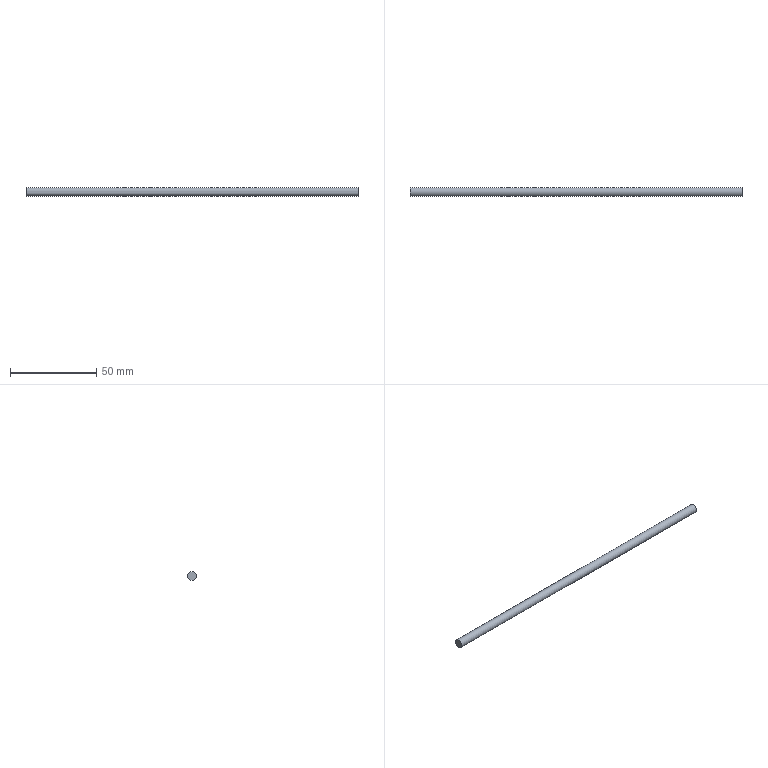Part | NX | features solid 2 | 1 solid | 3 faces | box 192 x 5 x 5 mm | volume 3770 mm3 | plane 2 | cylinder 1 | commonest cylinder face diameters 5 x1
STEP:
#1=CARTESIAN_POINT('',(-65.,-377.5,-412.5));
#2=VERTEX_POINT('',#1);
#3=CARTESIAN_POINT('',(-65.,-377.5,-410.));
#4=DIRECTION('',(1.,0.,0.));
#5=DIRECTION('',(0.,0.,-1.));
#6=AXIS2_PLACEMENT_3D('',#3,#4,#5);
#7=CIRCLE('',#6,2.5);
#8=EDGE_CURVE('',#2,#2,#7,.T.);
#9=ORIENTED_EDGE('',*,*,#8,.F.);
#10=EDGE_LOOP('',(#9));
#11=FACE_BOUND('',#10,.T.);
#12=CARTESIAN_POINT('',(-257.,-377.5,-412.5));
#13=VERTEX_POINT('',#12);
#14=CARTESIAN_POINT('',(-257.,-377.5,-410.));
#15=DIRECTION('',(1.,0.,0.));
#16=DIRECTION('',(0.,0.,-1.));
#17=AXIS2_PLACEMENT_3D('',#14,#15,#16);
#18=CIRCLE('',#17,2.5);
#19=EDGE_CURVE('',#13,#13,#18,.T.);
#20=ORIENTED_EDGE('',*,*,#19,.T.);
#21=EDGE_LOOP('',(#20));
#22=FACE_BOUND('',#21,.T.);
#23=CARTESIAN_POINT('',(-52.,-377.5,-410.));
#24=DIRECTION('',(-1.,0.,0.));
#25=DIRECTION('',(0.,0.,-1.));
#26=AXIS2_PLACEMENT_3D('',#23,#24,#25);
#27=CYLINDRICAL_SURFACE('',#26,2.5);
#28=ADVANCED_FACE('',(#11,#22),#27,.T.);
#29=ORIENTED_EDGE('',*,*,#8,.T.);
#30=EDGE_LOOP('',(#29));
#31=FACE_BOUND('',#30,.T.);
#32=CARTESIAN_POINT('',(-65.,80.624,-300.));
#33=DIRECTION('',(-1.,0.,0.));
#34=DIRECTION('',(0.,0.,-1.));
#35=AXIS2_PLACEMENT_3D('',#32,#33,#34);
#36=PLANE('',#35);
#37=ADVANCED_FACE('',(#31),#36,.F.);
#38=ORIENTED_EDGE('',*,*,#19,.F.);
#39=EDGE_LOOP('',(#38));
#40=FACE_BOUND('',#39,.T.);
#41=CARTESIAN_POINT('',(-257.,156.,-270.));
#42=DIRECTION('',(1.,0.,0.));
#43=DIRECTION('',(0.,0.,1.));
#44=AXIS2_PLACEMENT_3D('',#41,#42,#43);
#45=PLANE('',#44);
#46=ADVANCED_FACE('',(#40),#45,.F.);
#47=CLOSED_SHELL('',(#28,#37,#46));
#48=MANIFOLD_SOLID_BREP('',#47);
#49=(LENGTH_UNIT()NAMED_UNIT(*)SI_UNIT(.MILLI.,.METRE.));
#50=UNCERTAINTY_MEASURE_WITH_UNIT(LENGTH_MEASURE(0.00001),#49,'','');
#51=(NAMED_UNIT(*)PLANE_ANGLE_UNIT()SI_UNIT($,.RADIAN.));
#52=(NAMED_UNIT(*)SI_UNIT($,.STERADIAN.)SOLID_ANGLE_UNIT());
#53=(GEOMETRIC_REPRESENTATION_CONTEXT(3)GLOBAL_UNCERTAINTY_ASSIGNED_CONTEXT((#50))GLOBAL_UNIT_ASSIGNED_CONTEXT((#49,#51,#52))REPRESENTATION_CONTEXT('',''));
#54=ADVANCED_BREP_SHAPE_REPRESENTATION('',(#48),#53);